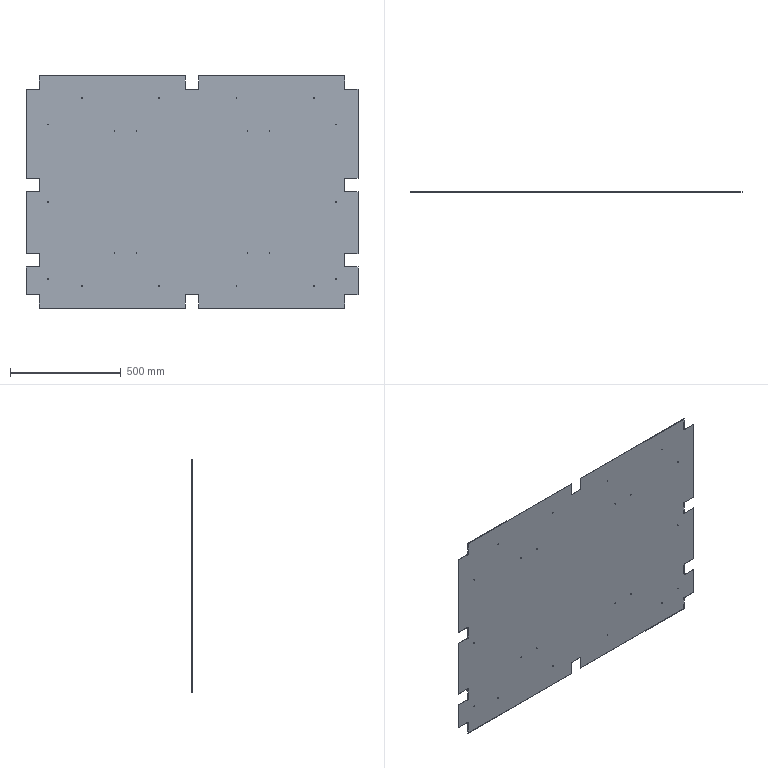Part | NX | features BREP 1 | 1 solid | 82 faces | box 1502 x 1.5 x 1050 mm | volume 2312494 mm3 | cylinder 44 | plane 38 | commonest cylinder face diameters 3.3 x44